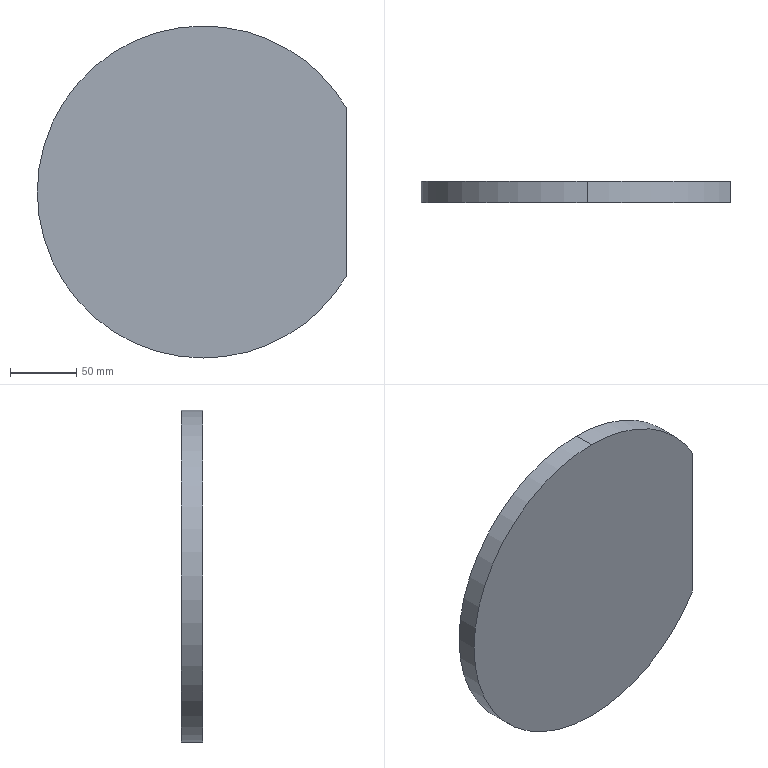Part | SolidWorks | features FlatPattern 1, SMBaseFlange 1, SheetMetal 1 | 1 solid | 6 faces | box 233 x 16 x 250 mm | volume 762244 mm3 | cylinder 3 | plane 3 | commonest cylinder face diameters 250 x3
STEP:
#1=CARTESIAN_POINT('',(0.,16.,125.));
#2=VERTEX_POINT('',#1);
#3=CARTESIAN_POINT('',(108.,16.,62.936));
#4=VERTEX_POINT('',#3);
#5=CARTESIAN_POINT('',(0.,16.,0.));
#6=DIRECTION('',(0.,1.,0.));
#7=DIRECTION('',(0.,0.,1.));
#8=AXIS2_PLACEMENT_3D('',#5,#6,#7);
#9=CIRCLE('',#8,125.);
#10=EDGE_CURVE('',#2,#4,#9,.T.);
#11=ORIENTED_EDGE('',*,*,#10,.F.);
#12=CARTESIAN_POINT('',(0.,0.,125.));
#13=VERTEX_POINT('',#12);
#14=CARTESIAN_POINT('',(0.,16.,125.));
#15=DIRECTION('',(0.,-1.,0.));
#16=VECTOR('',#15,1000.);
#17=LINE('',#14,#16);
#18=EDGE_CURVE('',#2,#13,#17,.T.);
#19=ORIENTED_EDGE('',*,*,#18,.T.);
#20=CARTESIAN_POINT('',(108.,0.,62.936));
#21=VERTEX_POINT('',#20);
#22=CARTESIAN_POINT('',(0.,0.,0.));
#23=DIRECTION('',(0.,1.,0.));
#24=DIRECTION('',(0.,0.,1.));
#25=AXIS2_PLACEMENT_3D('',#22,#23,#24);
#26=CIRCLE('',#25,125.);
#27=EDGE_CURVE('',#13,#21,#26,.T.);
#28=ORIENTED_EDGE('',*,*,#27,.T.);
#29=CARTESIAN_POINT('',(108.,16.,62.936));
#30=DIRECTION('',(0.,-1.,0.));
#31=VECTOR('',#30,1000.);
#32=LINE('',#29,#31);
#33=EDGE_CURVE('',#4,#21,#32,.T.);
#34=ORIENTED_EDGE('',*,*,#33,.F.);
#35=EDGE_LOOP('',(#11,#19,#28,#34));
#36=FACE_OUTER_BOUND('',#35,.T.);
#37=CARTESIAN_POINT('',(0.,16.,0.));
#38=DIRECTION('',(0.,-1.,0.));
#39=DIRECTION('',(0.,0.,-1.));
#40=AXIS2_PLACEMENT_3D('',#37,#38,#39);
#41=CYLINDRICAL_SURFACE('',#40,125.);
#42=ADVANCED_FACE('',(#36),#41,.T.);
#43=ORIENTED_EDGE('',*,*,#18,.F.);
#44=CARTESIAN_POINT('',(0.,16.,-125.));
#45=VERTEX_POINT('',#44);
#46=CARTESIAN_POINT('',(0.,16.,0.));
#47=DIRECTION('',(0.,1.,0.));
#48=DIRECTION('',(0.,0.,1.));
#49=AXIS2_PLACEMENT_3D('',#46,#47,#48);
#50=CIRCLE('',#49,125.);
#51=EDGE_CURVE('',#45,#2,#50,.T.);
#52=ORIENTED_EDGE('',*,*,#51,.F.);
#53=CARTESIAN_POINT('',(0.,0.,-125.));
#54=VERTEX_POINT('',#53);
#55=CARTESIAN_POINT('',(0.,16.,-125.));
#56=DIRECTION('',(0.,-1.,0.));
#57=VECTOR('',#56,1000.);
#58=LINE('',#55,#57);
#59=EDGE_CURVE('',#45,#54,#58,.T.);
#60=ORIENTED_EDGE('',*,*,#59,.T.);
#61=CARTESIAN_POINT('',(0.,0.,0.));
#62=DIRECTION('',(0.,1.,0.));
#63=DIRECTION('',(0.,0.,1.));
#64=AXIS2_PLACEMENT_3D('',#61,#62,#63);
#65=CIRCLE('',#64,125.);
#66=EDGE_CURVE('',#54,#13,#65,.T.);
#67=ORIENTED_EDGE('',*,*,#66,.T.);
#68=EDGE_LOOP('',(#43,#52,#60,#67));
#69=FACE_OUTER_BOUND('',#68,.T.);
#70=CARTESIAN_POINT('',(0.,16.,0.));
#71=DIRECTION('',(0.,-1.,0.));
#72=DIRECTION('',(0.,0.,-1.));
#73=AXIS2_PLACEMENT_3D('',#70,#71,#72);
#74=CYLINDRICAL_SURFACE('',#73,125.);
#75=ADVANCED_FACE('',(#69),#74,.T.);
#76=ORIENTED_EDGE('',*,*,#59,.F.);
#77=CARTESIAN_POINT('',(108.,16.,-62.936));
#78=VERTEX_POINT('',#77);
#79=CARTESIAN_POINT('',(0.,16.,0.));
#80=DIRECTION('',(0.,1.,0.));
#81=DIRECTION('',(0.,0.,1.));
#82=AXIS2_PLACEMENT_3D('',#79,#80,#81);
#83=CIRCLE('',#82,125.);
#84=EDGE_CURVE('',#78,#45,#83,.T.);
#85=ORIENTED_EDGE('',*,*,#84,.F.);
#86=CARTESIAN_POINT('',(108.,0.,-62.936));
#87=VERTEX_POINT('',#86);
#88=CARTESIAN_POINT('',(108.,16.,-62.936));
#89=DIRECTION('',(0.,-1.,0.));
#90=VECTOR('',#89,1000.);
#91=LINE('',#88,#90);
#92=EDGE_CURVE('',#78,#87,#91,.T.);
#93=ORIENTED_EDGE('',*,*,#92,.T.);
#94=CARTESIAN_POINT('',(0.,0.,0.));
#95=DIRECTION('',(0.,1.,0.));
#96=DIRECTION('',(0.,0.,1.));
#97=AXIS2_PLACEMENT_3D('',#94,#95,#96);
#98=CIRCLE('',#97,125.);
#99=EDGE_CURVE('',#87,#54,#98,.T.);
#100=ORIENTED_EDGE('',*,*,#99,.T.);
#101=EDGE_LOOP('',(#76,#85,#93,#100));
#102=FACE_OUTER_BOUND('',#101,.T.);
#103=CARTESIAN_POINT('',(0.,16.,0.));
#104=DIRECTION('',(0.,-1.,0.));
#105=DIRECTION('',(0.,0.,-1.));
#106=AXIS2_PLACEMENT_3D('',#103,#104,#105);
#107=CYLINDRICAL_SURFACE('',#106,125.);
#108=ADVANCED_FACE('',(#102),#107,.T.);
#109=CARTESIAN_POINT('',(108.,0.,-62.936));
#110=DIRECTION('',(0.,0.,-1.));
#111=VECTOR('',#110,1000.);
#112=LINE('',#109,#111);
#113=EDGE_CURVE('',#21,#87,#112,.T.);
#114=ORIENTED_EDGE('',*,*,#113,.T.);
#115=ORIENTED_EDGE('',*,*,#92,.F.);
#116=CARTESIAN_POINT('',(108.,16.,-62.936));
#117=DIRECTION('',(0.,0.,-1.));
#118=VECTOR('',#117,1000.);
#119=LINE('',#116,#118);
#120=EDGE_CURVE('',#4,#78,#119,.T.);
#121=ORIENTED_EDGE('',*,*,#120,.F.);
#122=ORIENTED_EDGE('',*,*,#33,.T.);
#123=EDGE_LOOP('',(#114,#115,#121,#122));
#124=FACE_OUTER_BOUND('',#123,.T.);
#125=CARTESIAN_POINT('',(108.,16.,-62.936));
#126=DIRECTION('',(-1.,0.,0.));
#127=DIRECTION('',(0.,0.,1.));
#128=AXIS2_PLACEMENT_3D('',#125,#126,#127);
#129=PLANE('',#128);
#130=ADVANCED_FACE('',(#124),#129,.F.);
#131=ORIENTED_EDGE('',*,*,#84,.T.);
#132=ORIENTED_EDGE('',*,*,#51,.T.);
#133=ORIENTED_EDGE('',*,*,#10,.T.);
#134=ORIENTED_EDGE('',*,*,#120,.T.);
#135=EDGE_LOOP('',(#131,#132,#133,#134));
#136=FACE_OUTER_BOUND('',#135,.T.);
#137=CARTESIAN_POINT('',(0.,16.,0.));
#138=DIRECTION('',(0.,1.,0.));
#139=DIRECTION('',(0.,0.,1.));
#140=AXIS2_PLACEMENT_3D('',#137,#138,#139);
#141=PLANE('',#140);
#142=ADVANCED_FACE('',(#136),#141,.T.);
#143=ORIENTED_EDGE('',*,*,#99,.F.);
#144=ORIENTED_EDGE('',*,*,#113,.F.);
#145=ORIENTED_EDGE('',*,*,#27,.F.);
#146=ORIENTED_EDGE('',*,*,#66,.F.);
#147=EDGE_LOOP('',(#143,#144,#145,#146));
#148=FACE_OUTER_BOUND('',#147,.T.);
#149=CARTESIAN_POINT('',(0.,0.,0.));
#150=DIRECTION('',(0.,1.,0.));
#151=DIRECTION('',(0.,0.,1.));
#152=AXIS2_PLACEMENT_3D('',#149,#150,#151);
#153=PLANE('',#152);
#154=ADVANCED_FACE('',(#148),#153,.F.);
#155=CLOSED_SHELL('',(#42,#75,#108,#130,#142,#154));
#156=MANIFOLD_SOLID_BREP('',#155);
#157=CARTESIAN_POINT('',(0.,0.,0.));
#158=DIRECTION('',(0.,0.,1.));
#159=DIRECTION('',(1.,0.,0.));
#160=AXIS2_PLACEMENT_3D('',#157,#158,#159);
#161=(LENGTH_UNIT()NAMED_UNIT(*)SI_UNIT(.MILLI.,.METRE.));
#162=UNCERTAINTY_MEASURE_WITH_UNIT(LENGTH_MEASURE(0.00001),#161,'','');
#163=(NAMED_UNIT(*)PLANE_ANGLE_UNIT()SI_UNIT($,.RADIAN.));
#164=(NAMED_UNIT(*)SI_UNIT($,.STERADIAN.)SOLID_ANGLE_UNIT());
#165=(GEOMETRIC_REPRESENTATION_CONTEXT(3)GLOBAL_UNCERTAINTY_ASSIGNED_CONTEXT((#162))GLOBAL_UNIT_ASSIGNED_CONTEXT((#161,#163,#164))REPRESENTATION_CONTEXT('',''));
#166=ADVANCED_BREP_SHAPE_REPRESENTATION('',(#156,#160),#165);